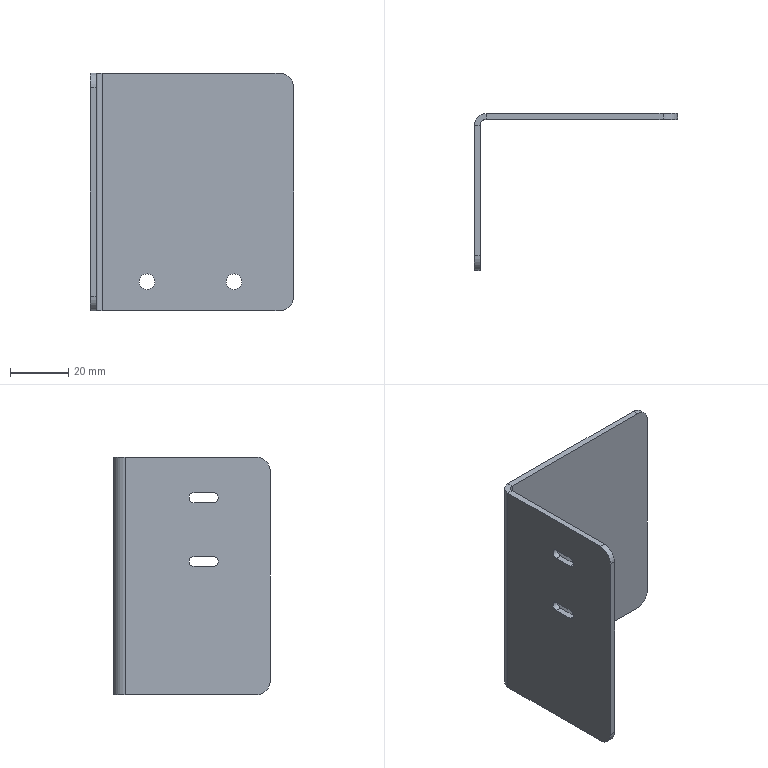Part | SolidWorks | features HoleWzd 3, EdgeFlange 2, Chamfer 1, Fillet 1, FlatPattern 1, MirrorPattern 1, SMBaseFlange 1, SheetMetal 1 | 1 solid | 30 faces | box 70 x 54 x 82 mm | volume 19533 mm3 | plane 16 | cylinder 14 | commonest cylinder face diameters 3.4 x4 5.5 x4 10 x4 4 x1 8 x1
STEP:
#1=CARTESIAN_POINT('',(47.503,28.,-28.25));
#2=VERTEX_POINT('',#1);
#3=CARTESIAN_POINT('',(47.503,28.,-33.75));
#4=VERTEX_POINT('',#3);
#5=CARTESIAN_POINT('',(47.503,28.,-31.));
#6=DIRECTION('',(0.,-1.,0.));
#7=DIRECTION('',(0.,0.,-1.));
#8=AXIS2_PLACEMENT_3D('',#5,#6,#7);
#9=CIRCLE('',#8,2.75);
#10=EDGE_CURVE('',#2,#4,#9,.T.);
#11=ORIENTED_EDGE('',*,*,#10,.F.);
#12=CARTESIAN_POINT('',(47.503,26.,-28.25));
#13=VERTEX_POINT('',#12);
#14=CARTESIAN_POINT('',(47.503,26.,-28.25));
#15=DIRECTION('',(0.,-1.,0.));
#16=VECTOR('',#15,1000.);
#17=LINE('',#14,#16);
#18=EDGE_CURVE('',#2,#13,#17,.T.);
#19=ORIENTED_EDGE('',*,*,#18,.T.);
#20=CARTESIAN_POINT('',(47.503,26.,-33.75));
#21=VERTEX_POINT('',#20);
#22=CARTESIAN_POINT('',(47.503,26.,-31.));
#23=DIRECTION('',(0.,-1.,0.));
#24=DIRECTION('',(0.,0.,-1.));
#25=AXIS2_PLACEMENT_3D('',#22,#23,#24);
#26=CIRCLE('',#25,2.75);
#27=EDGE_CURVE('',#13,#21,#26,.T.);
#28=ORIENTED_EDGE('',*,*,#27,.T.);
#29=CARTESIAN_POINT('',(47.503,26.,-33.75));
#30=DIRECTION('',(0.,-1.,0.));
#31=VECTOR('',#30,1000.);
#32=LINE('',#29,#31);
#33=EDGE_CURVE('',#4,#21,#32,.T.);
#34=ORIENTED_EDGE('',*,*,#33,.F.);
#35=EDGE_LOOP('',(#11,#19,#28,#34));
#36=FACE_OUTER_BOUND('',#35,.T.);
#37=CARTESIAN_POINT('',(47.503,26.,-31.));
#38=DIRECTION('',(0.,-1.,0.));
#39=DIRECTION('',(0.,0.,-1.));
#40=AXIS2_PLACEMENT_3D('',#37,#38,#39);
#41=CYLINDRICAL_SURFACE('',#40,2.75);
#42=ADVANCED_FACE('',(#36),#41,.F.);
#43=CARTESIAN_POINT('',(17.503,28.,-28.25));
#44=VERTEX_POINT('',#43);
#45=CARTESIAN_POINT('',(17.503,28.,-33.75));
#46=VERTEX_POINT('',#45);
#47=CARTESIAN_POINT('',(17.503,28.,-31.));
#48=DIRECTION('',(0.,-1.,0.));
#49=DIRECTION('',(0.,0.,-1.));
#50=AXIS2_PLACEMENT_3D('',#47,#48,#49);
#51=CIRCLE('',#50,2.75);
#52=EDGE_CURVE('',#44,#46,#51,.T.);
#53=ORIENTED_EDGE('',*,*,#52,.F.);
#54=CARTESIAN_POINT('',(17.503,26.,-28.25));
#55=VERTEX_POINT('',#54);
#56=CARTESIAN_POINT('',(17.503,26.,-28.25));
#57=DIRECTION('',(0.,-1.,0.));
#58=VECTOR('',#57,1000.);
#59=LINE('',#56,#58);
#60=EDGE_CURVE('',#44,#55,#59,.T.);
#61=ORIENTED_EDGE('',*,*,#60,.T.);
#62=CARTESIAN_POINT('',(17.503,26.,-33.75));
#63=VERTEX_POINT('',#62);
#64=CARTESIAN_POINT('',(17.503,26.,-31.));
#65=DIRECTION('',(0.,-1.,0.));
#66=DIRECTION('',(0.,0.,-1.));
#67=AXIS2_PLACEMENT_3D('',#64,#65,#66);
#68=CIRCLE('',#67,2.75);
#69=EDGE_CURVE('',#55,#63,#68,.T.);
#70=ORIENTED_EDGE('',*,*,#69,.T.);
#71=CARTESIAN_POINT('',(17.503,26.,-33.75));
#72=DIRECTION('',(0.,-1.,0.));
#73=VECTOR('',#72,1000.);
#74=LINE('',#71,#73);
#75=EDGE_CURVE('',#46,#63,#74,.T.);
#76=ORIENTED_EDGE('',*,*,#75,.F.);
#77=EDGE_LOOP('',(#53,#61,#70,#76));
#78=FACE_OUTER_BOUND('',#77,.T.);
#79=CARTESIAN_POINT('',(17.503,26.,-31.));
#80=DIRECTION('',(0.,-1.,0.));
#81=DIRECTION('',(0.,0.,-1.));
#82=AXIS2_PLACEMENT_3D('',#79,#80,#81);
#83=CYLINDRICAL_SURFACE('',#82,2.75);
#84=ADVANCED_FACE('',(#78),#83,.F.);
#85=CARTESIAN_POINT('',(-2.,24.,41.));
#86=VERTEX_POINT('',#85);
#87=CARTESIAN_POINT('',(-2.,-21.,41.));
#88=VERTEX_POINT('',#87);
#89=CARTESIAN_POINT('',(-2.,26.,41.));
#90=DIRECTION('',(0.,-1.,0.));
#91=VECTOR('',#90,1000.);
#92=LINE('',#89,#91);
#93=EDGE_CURVE('',#86,#88,#92,.T.);
#94=ORIENTED_EDGE('',*,*,#93,.T.);
#95=CARTESIAN_POINT('',(0.,-21.,41.));
#96=VERTEX_POINT('',#95);
#97=CARTESIAN_POINT('',(-2.,-21.,41.));
#98=DIRECTION('',(1.,0.,0.));
#99=VECTOR('',#98,1000.);
#100=LINE('',#97,#99);
#101=EDGE_CURVE('',#88,#96,#100,.T.);
#102=ORIENTED_EDGE('',*,*,#101,.T.);
#103=CARTESIAN_POINT('',(0.,24.,41.));
#104=VERTEX_POINT('',#103);
#105=CARTESIAN_POINT('',(0.,26.,41.));
#106=DIRECTION('',(0.,-1.,0.));
#107=VECTOR('',#106,1000.);
#108=LINE('',#105,#107);
#109=EDGE_CURVE('',#104,#96,#108,.T.);
#110=ORIENTED_EDGE('',*,*,#109,.F.);
#111=CARTESIAN_POINT('',(0.,24.,41.));
#112=DIRECTION('',(-1.,0.,0.));
#113=VECTOR('',#112,1000.);
#114=LINE('',#111,#113);
#115=EDGE_CURVE('',#104,#86,#114,.T.);
#116=ORIENTED_EDGE('',*,*,#115,.T.);
#117=EDGE_LOOP('',(#94,#102,#110,#116));
#118=FACE_OUTER_BOUND('',#117,.T.);
#119=CARTESIAN_POINT('',(-2.,26.,41.));
#120=DIRECTION('',(0.,0.,1.));
#121=DIRECTION('',(0.,-1.,0.));
#122=AXIS2_PLACEMENT_3D('',#119,#120,#121);
#123=PLANE('',#122);
#124=ADVANCED_FACE('',(#118),#123,.T.);
#125=CARTESIAN_POINT('',(-2.,-6.3,6.7));
#126=VERTEX_POINT('',#125);
#127=CARTESIAN_POINT('',(-2.,-6.3,3.3));
#128=VERTEX_POINT('',#127);
#129=CARTESIAN_POINT('',(-2.,-6.3,5.));
#130=DIRECTION('',(1.,0.,0.));
#131=DIRECTION('',(0.,0.,-1.));
#132=AXIS2_PLACEMENT_3D('',#129,#130,#131);
#133=CIRCLE('',#132,1.7);
#134=EDGE_CURVE('',#126,#128,#133,.T.);
#135=ORIENTED_EDGE('',*,*,#134,.T.);
#136=CARTESIAN_POINT('',(-2.,0.3,3.3));
#137=VERTEX_POINT('',#136);
#138=CARTESIAN_POINT('',(-2.,-6.3,3.3));
#139=DIRECTION('',(0.,1.,0.));
#140=VECTOR('',#139,1000.);
#141=LINE('',#138,#140);
#142=EDGE_CURVE('',#128,#137,#141,.T.);
#143=ORIENTED_EDGE('',*,*,#142,.T.);
#144=CARTESIAN_POINT('',(-2.,0.3,6.7));
#145=VERTEX_POINT('',#144);
#146=CARTESIAN_POINT('',(-2.,0.3,5.));
#147=DIRECTION('',(1.,0.,0.));
#148=DIRECTION('',(0.,0.,-1.));
#149=AXIS2_PLACEMENT_3D('',#146,#147,#148);
#150=CIRCLE('',#149,1.7);
#151=EDGE_CURVE('',#137,#145,#150,.T.);
#152=ORIENTED_EDGE('',*,*,#151,.T.);
#153=CARTESIAN_POINT('',(-2.,-6.3,6.7));
#154=DIRECTION('',(0.,1.,0.));
#155=VECTOR('',#154,1000.);
#156=LINE('',#153,#155);
#157=EDGE_CURVE('',#126,#145,#156,.T.);
#158=ORIENTED_EDGE('',*,*,#157,.F.);
#159=EDGE_LOOP('',(#135,#143,#152,#158));
#160=FACE_BOUND('',#159,.T.);
#161=CARTESIAN_POINT('',(-2.,-6.3,25.3));
#162=VERTEX_POINT('',#161);
#163=CARTESIAN_POINT('',(-2.,0.3,25.3));
#164=VERTEX_POINT('',#163);
#165=CARTESIAN_POINT('',(-2.,-6.3,25.3));
#166=DIRECTION('',(0.,1.,0.));
#167=VECTOR('',#166,1000.);
#168=LINE('',#165,#167);
#169=EDGE_CURVE('',#162,#164,#168,.T.);
#170=ORIENTED_EDGE('',*,*,#169,.T.);
#171=CARTESIAN_POINT('',(-2.,0.3,28.7));
#172=VERTEX_POINT('',#171);
#173=CARTESIAN_POINT('',(-2.,0.3,27.));
#174=DIRECTION('',(1.,0.,0.));
#175=DIRECTION('',(0.,0.,-1.));
#176=AXIS2_PLACEMENT_3D('',#173,#174,#175);
#177=CIRCLE('',#176,1.7);
#178=EDGE_CURVE('',#164,#172,#177,.T.);
#179=ORIENTED_EDGE('',*,*,#178,.T.);
#180=CARTESIAN_POINT('',(-2.,-6.3,28.7));
#181=VERTEX_POINT('',#180);
#182=CARTESIAN_POINT('',(-2.,-6.3,28.7));
#183=DIRECTION('',(0.,1.,0.));
#184=VECTOR('',#183,1000.);
#185=LINE('',#182,#184);
#186=EDGE_CURVE('',#181,#172,#185,.T.);
#187=ORIENTED_EDGE('',*,*,#186,.F.);
#188=CARTESIAN_POINT('',(-2.,-6.3,27.));
#189=DIRECTION('',(1.,0.,0.));
#190=DIRECTION('',(0.,0.,-1.));
#191=AXIS2_PLACEMENT_3D('',#188,#189,#190);
#192=CIRCLE('',#191,1.7);
#193=EDGE_CURVE('',#181,#162,#192,.T.);
#194=ORIENTED_EDGE('',*,*,#193,.T.);
#195=EDGE_LOOP('',(#170,#179,#187,#194));
#196=FACE_BOUND('',#195,.T.);
#197=CARTESIAN_POINT('',(-2.,-21.,-41.));
#198=VERTEX_POINT('',#197);
#199=CARTESIAN_POINT('',(-2.,24.,-41.));
#200=VERTEX_POINT('',#199);
#201=CARTESIAN_POINT('',(-2.,26.,-41.));
#202=DIRECTION('',(0.,1.,0.));
#203=VECTOR('',#202,1000.);
#204=LINE('',#201,#203);
#205=EDGE_CURVE('',#198,#200,#204,.T.);
#206=ORIENTED_EDGE('',*,*,#205,.F.);
#207=CARTESIAN_POINT('',(-2.,-26.,-36.));
#208=VERTEX_POINT('',#207);
#209=CARTESIAN_POINT('',(-2.,-21.,-36.));
#210=DIRECTION('',(-1.,0.,0.));
#211=DIRECTION('',(0.,0.,-1.));
#212=AXIS2_PLACEMENT_3D('',#209,#210,#211);
#213=CIRCLE('',#212,5.);
#214=EDGE_CURVE('',#198,#208,#213,.T.);
#215=ORIENTED_EDGE('',*,*,#214,.T.);
#216=CARTESIAN_POINT('',(-2.,-26.,36.));
#217=VERTEX_POINT('',#216);
#218=CARTESIAN_POINT('',(-2.,-26.,41.));
#219=DIRECTION('',(0.,0.,-1.));
#220=VECTOR('',#219,1000.);
#221=LINE('',#218,#220);
#222=EDGE_CURVE('',#217,#208,#221,.T.);
#223=ORIENTED_EDGE('',*,*,#222,.F.);
#224=CARTESIAN_POINT('',(-2.,-21.,36.));
#225=DIRECTION('',(-1.,0.,0.));
#226=DIRECTION('',(0.,0.,-1.));
#227=AXIS2_PLACEMENT_3D('',#224,#225,#226);
#228=CIRCLE('',#227,5.);
#229=EDGE_CURVE('',#217,#88,#228,.T.);
#230=ORIENTED_EDGE('',*,*,#229,.T.);
#231=ORIENTED_EDGE('',*,*,#93,.F.);
#232=CARTESIAN_POINT('',(-2.,24.,41.));
#233=DIRECTION('',(0.,0.,-1.));
#234=VECTOR('',#233,1000.);
#235=LINE('',#232,#234);
#236=EDGE_CURVE('',#86,#200,#235,.T.);
#237=ORIENTED_EDGE('',*,*,#236,.T.);
#238=EDGE_LOOP('',(#206,#215,#223,#230,#231,#237));
#239=FACE_OUTER_BOUND('',#238,.T.);
#240=CARTESIAN_POINT('',(-2.,0.,0.));
#241=DIRECTION('',(1.,0.,0.));
#242=DIRECTION('',(0.,0.,-1.));
#243=AXIS2_PLACEMENT_3D('',#240,#241,#242);
#244=PLANE('',#243);
#245=ADVANCED_FACE('',(#160,#196,#239),#244,.F.);
#246=CARTESIAN_POINT('',(0.,0.3,25.3));
#247=VERTEX_POINT('',#246);
#248=CARTESIAN_POINT('',(0.,0.3,28.7));
#249=VERTEX_POINT('',#248);
#250=CARTESIAN_POINT('',(0.,0.3,27.));
#251=DIRECTION('',(1.,0.,0.));
#252=DIRECTION('',(0.,0.,-1.));
#253=AXIS2_PLACEMENT_3D('',#250,#251,#252);
#254=CIRCLE('',#253,1.7);
#255=EDGE_CURVE('',#247,#249,#254,.T.);
#256=ORIENTED_EDGE('',*,*,#255,.F.);
#257=CARTESIAN_POINT('',(0.,-6.3,25.3));
#258=VERTEX_POINT('',#257);
#259=CARTESIAN_POINT('',(0.,-6.3,25.3));
#260=DIRECTION('',(0.,1.,0.));
#261=VECTOR('',#260,1000.);
#262=LINE('',#259,#261);
#263=EDGE_CURVE('',#258,#247,#262,.T.);
#264=ORIENTED_EDGE('',*,*,#263,.F.);
#265=CARTESIAN_POINT('',(0.,-6.3,28.7));
#266=VERTEX_POINT('',#265);
#267=CARTESIAN_POINT('',(0.,-6.3,27.));
#268=DIRECTION('',(1.,0.,0.));
#269=DIRECTION('',(0.,0.,-1.));
#270=AXIS2_PLACEMENT_3D('',#267,#268,#269);
#271=CIRCLE('',#270,1.7);
#272=EDGE_CURVE('',#266,#258,#271,.T.);
#273=ORIENTED_EDGE('',*,*,#272,.F.);
#274=CARTESIAN_POINT('',(0.,-6.3,28.7));
#275=DIRECTION('',(0.,1.,0.));
#276=VECTOR('',#275,1000.);
#277=LINE('',#274,#276);
#278=EDGE_CURVE('',#266,#249,#277,.T.);
#279=ORIENTED_EDGE('',*,*,#278,.T.);
#280=EDGE_LOOP('',(#256,#264,#273,#279));
#281=FACE_BOUND('',#280,.T.);
#282=CARTESIAN_POINT('',(0.,-6.3,3.3));
#283=VERTEX_POINT('',#282);
#284=CARTESIAN_POINT('',(0.,0.3,3.3));
#285=VERTEX_POINT('',#284);
#286=CARTESIAN_POINT('',(0.,-6.3,3.3));
#287=DIRECTION('',(0.,1.,0.));
#288=VECTOR('',#287,1000.);
#289=LINE('',#286,#288);
#290=EDGE_CURVE('',#283,#285,#289,.T.);
#291=ORIENTED_EDGE('',*,*,#290,.F.);
#292=CARTESIAN_POINT('',(0.,-6.3,6.7));
#293=VERTEX_POINT('',#292);
#294=CARTESIAN_POINT('',(0.,-6.3,5.));
#295=DIRECTION('',(1.,0.,0.));
#296=DIRECTION('',(0.,0.,-1.));
#297=AXIS2_PLACEMENT_3D('',#294,#295,#296);
#298=CIRCLE('',#297,1.7);
#299=EDGE_CURVE('',#293,#283,#298,.T.);
#300=ORIENTED_EDGE('',*,*,#299,.F.);
#301=CARTESIAN_POINT('',(0.,0.3,6.7));
#302=VERTEX_POINT('',#301);
#303=CARTESIAN_POINT('',(0.,-6.3,6.7));
#304=DIRECTION('',(0.,1.,0.));
#305=VECTOR('',#304,1000.);
#306=LINE('',#303,#305);
#307=EDGE_CURVE('',#293,#302,#306,.T.);
#308=ORIENTED_EDGE('',*,*,#307,.T.);
#309=CARTESIAN_POINT('',(0.,0.3,5.));
#310=DIRECTION('',(1.,0.,0.));
#311=DIRECTION('',(0.,0.,-1.));
#312=AXIS2_PLACEMENT_3D('',#309,#310,#311);
#313=CIRCLE('',#312,1.7);
#314=EDGE_CURVE('',#285,#302,#313,.T.);
#315=ORIENTED_EDGE('',*,*,#314,.F.);
#316=EDGE_LOOP('',(#291,#300,#308,#315));
#317=FACE_BOUND('',#316,.T.);
#318=CARTESIAN_POINT('',(0.,-26.,36.));
#319=VERTEX_POINT('',#318);
#320=CARTESIAN_POINT('',(0.,-26.,-36.));
#321=VERTEX_POINT('',#320);
#322=CARTESIAN_POINT('',(0.,-26.,41.));
#323=DIRECTION('',(0.,0.,-1.));
#324=VECTOR('',#323,1000.);
#325=LINE('',#322,#324);
#326=EDGE_CURVE('',#319,#321,#325,.T.);
#327=ORIENTED_EDGE('',*,*,#326,.T.);
#328=CARTESIAN_POINT('',(0.,-21.,-41.));
#329=VERTEX_POINT('',#328);
#330=CARTESIAN_POINT('',(0.,-21.,-36.));
#331=DIRECTION('',(1.,0.,0.));
#332=DIRECTION('',(0.,0.,-1.));
#333=AXIS2_PLACEMENT_3D('',#330,#331,#332);
#334=CIRCLE('',#333,5.);
#335=EDGE_CURVE('',#321,#329,#334,.T.);
#336=ORIENTED_EDGE('',*,*,#335,.T.);
#337=CARTESIAN_POINT('',(0.,24.,-41.));
#338=VERTEX_POINT('',#337);
#339=CARTESIAN_POINT('',(0.,26.,-41.));
#340=DIRECTION('',(0.,1.,0.));
#341=VECTOR('',#340,1000.);
#342=LINE('',#339,#341);
#343=EDGE_CURVE('',#329,#338,#342,.T.);
#344=ORIENTED_EDGE('',*,*,#343,.T.);
#345=CARTESIAN_POINT('',(0.,24.,41.));
#346=DIRECTION('',(0.,0.,-1.));
#347=VECTOR('',#346,1000.);
#348=LINE('',#345,#347);
#349=EDGE_CURVE('',#104,#338,#348,.T.);
#350=ORIENTED_EDGE('',*,*,#349,.F.);
#351=ORIENTED_EDGE('',*,*,#109,.T.);
#352=CARTESIAN_POINT('',(0.,-21.,36.));
#353=DIRECTION('',(1.,0.,0.));
#354=DIRECTION('',(0.,0.,-1.));
#355=AXIS2_PLACEMENT_3D('',#352,#353,#354);
#356=CIRCLE('',#355,5.);
#357=EDGE_CURVE('',#96,#319,#356,.T.);
#358=ORIENTED_EDGE('',*,*,#357,.T.);
#359=EDGE_LOOP('',(#327,#336,#344,#350,#351,#358));
#360=FACE_OUTER_BOUND('',#359,.T.);
#361=CARTESIAN_POINT('',(0.,0.,0.));
#362=DIRECTION('',(1.,0.,0.));
#363=DIRECTION('',(0.,0.,-1.));
#364=AXIS2_PLACEMENT_3D('',#361,#362,#363);
#365=PLANE('',#364);
#366=ADVANCED_FACE('',(#281,#317,#360),#365,.T.);
#367=ORIENTED_EDGE('',*,*,#343,.F.);
#368=CARTESIAN_POINT('',(-2.,-21.,-41.));
#369=DIRECTION('',(-1.,0.,0.));
#370=VECTOR('',#369,1000.);
#371=LINE('',#368,#370);
#372=EDGE_CURVE('',#329,#198,#371,.T.);
#373=ORIENTED_EDGE('',*,*,#372,.T.);
#374=ORIENTED_EDGE('',*,*,#205,.T.);
#375=CARTESIAN_POINT('',(0.,24.,-41.));
#376=DIRECTION('',(-1.,0.,0.));
#377=VECTOR('',#376,1000.);
#378=LINE('',#375,#377);
#379=EDGE_CURVE('',#338,#200,#378,.T.);
#380=ORIENTED_EDGE('',*,*,#379,.F.);
#381=EDGE_LOOP('',(#367,#373,#374,#380));
#382=FACE_OUTER_BOUND('',#381,.T.);
#383=CARTESIAN_POINT('',(-2.,26.,-41.));
#384=DIRECTION('',(0.,0.,-1.));
#385=DIRECTION('',(0.,1.,0.));
#386=AXIS2_PLACEMENT_3D('',#383,#384,#385);
#387=PLANE('',#386);
#388=ADVANCED_FACE('',(#382),#387,.T.);
#389=ORIENTED_EDGE('',*,*,#222,.T.);
#390=CARTESIAN_POINT('',(-2.,-26.,-36.));
#391=DIRECTION('',(1.,0.,0.));
#392=VECTOR('',#391,1000.);
#393=LINE('',#390,#392);
#394=EDGE_CURVE('',#208,#321,#393,.T.);
#395=ORIENTED_EDGE('',*,*,#394,.T.);
#396=ORIENTED_EDGE('',*,*,#326,.F.);
#397=CARTESIAN_POINT('',(-2.,-26.,36.));
#398=DIRECTION('',(-1.,0.,0.));
#399=VECTOR('',#398,1000.);
#400=LINE('',#397,#399);
#401=EDGE_CURVE('',#319,#217,#400,.T.);
#402=ORIENTED_EDGE('',*,*,#401,.T.);
#403=EDGE_LOOP('',(#389,#395,#396,#402));
#404=FACE_OUTER_BOUND('',#403,.T.);
#405=CARTESIAN_POINT('',(-2.,-26.,41.));
#406=DIRECTION('',(0.,-1.,0.));
#407=DIRECTION('',(0.,0.,-1.));
#408=AXIS2_PLACEMENT_3D('',#405,#406,#407);
#409=PLANE('',#408);
#410=ADVANCED_FACE('',(#404),#409,.T.);
#411=ORIENTED_EDGE('',*,*,#151,.F.);
#412=CARTESIAN_POINT('',(0.,0.3,3.3));
#413=DIRECTION('',(-1.,0.,0.));
#414=VECTOR('',#413,1000.);
#415=LINE('',#412,#414);
#416=EDGE_CURVE('',#285,#137,#415,.T.);
#417=ORIENTED_EDGE('',*,*,#416,.F.);
#418=ORIENTED_EDGE('',*,*,#314,.T.);
#419=CARTESIAN_POINT('',(0.,0.3,6.7));
#420=DIRECTION('',(1.,0.,0.));
#421=VECTOR('',#420,1000.);
#422=LINE('',#419,#421);
#423=EDGE_CURVE('',#145,#302,#422,.T.);
#424=ORIENTED_EDGE('',*,*,#423,.F.);
#425=EDGE_LOOP('',(#411,#417,#418,#424));
#426=FACE_OUTER_BOUND('',#425,.T.);
#427=CARTESIAN_POINT('',(0.,0.3,5.));
#428=DIRECTION('',(1.,0.,0.));
#429=DIRECTION('',(0.,0.,-1.));
#430=AXIS2_PLACEMENT_3D('',#427,#428,#429);
#431=CYLINDRICAL_SURFACE('',#430,1.7);
#432=ADVANCED_FACE('',(#426),#431,.F.);
#433=ORIENTED_EDGE('',*,*,#299,.T.);
#434=CARTESIAN_POINT('',(0.,-6.3,3.3));
#435=DIRECTION('',(1.,0.,0.));
#436=VECTOR('',#435,1000.);
#437=LINE('',#434,#436);
#438=EDGE_CURVE('',#128,#283,#437,.T.);
#439=ORIENTED_EDGE('',*,*,#438,.F.);
#440=ORIENTED_EDGE('',*,*,#134,.F.);
#441=CARTESIAN_POINT('',(0.,-6.3,6.7));
#442=DIRECTION('',(-1.,0.,0.));
#443=VECTOR('',#442,1000.);
#444=LINE('',#441,#443);
#445=EDGE_CURVE('',#293,#126,#444,.T.);
#446=ORIENTED_EDGE('',*,*,#445,.F.);
#447=EDGE_LOOP('',(#433,#439,#440,#446));
#448=FACE_OUTER_BOUND('',#447,.T.);
#449=CARTESIAN_POINT('',(0.,-6.3,5.));
#450=DIRECTION('',(1.,0.,0.));
#451=DIRECTION('',(0.,0.,-1.));
#452=AXIS2_PLACEMENT_3D('',#449,#450,#451);
#453=CYLINDRICAL_SURFACE('',#452,1.7);
#454=ADVANCED_FACE('',(#448),#453,.F.);
#455=ORIENTED_EDGE('',*,*,#423,.T.);
#456=ORIENTED_EDGE('',*,*,#307,.F.);
#457=ORIENTED_EDGE('',*,*,#445,.T.);
#458=ORIENTED_EDGE('',*,*,#157,.T.);
#459=EDGE_LOOP('',(#455,#456,#457,#458));
#460=FACE_OUTER_BOUND('',#459,.T.);
#461=CARTESIAN_POINT('',(0.,-6.3,6.7));
#462=DIRECTION('',(0.,0.,1.));
#463=DIRECTION('',(1.,0.,0.));
#464=AXIS2_PLACEMENT_3D('',#461,#462,#463);
#465=PLANE('',#464);
#466=ADVANCED_FACE('',(#460),#465,.F.);
#467=ORIENTED_EDGE('',*,*,#416,.T.);
#468=ORIENTED_EDGE('',*,*,#142,.F.);
#469=ORIENTED_EDGE('',*,*,#438,.T.);
#470=ORIENTED_EDGE('',*,*,#290,.T.);
#471=EDGE_LOOP('',(#467,#468,#469,#470));
#472=FACE_OUTER_BOUND('',#471,.T.);
#473=CARTESIAN_POINT('',(0.,-6.3,3.3));
#474=DIRECTION('',(0.,0.,-1.));
#475=DIRECTION('',(-1.,0.,0.));
#476=AXIS2_PLACEMENT_3D('',#473,#474,#475);
#477=PLANE('',#476);
#478=ADVANCED_FACE('',(#472),#477,.F.);
#479=ORIENTED_EDGE('',*,*,#178,.F.);
#480=CARTESIAN_POINT('',(0.,0.3,25.3));
#481=DIRECTION('',(-1.,0.,0.));
#482=VECTOR('',#481,1000.);
#483=LINE('',#480,#482);
#484=EDGE_CURVE('',#247,#164,#483,.T.);
#485=ORIENTED_EDGE('',*,*,#484,.F.);
#486=ORIENTED_EDGE('',*,*,#255,.T.);
#487=CARTESIAN_POINT('',(0.,0.3,28.7));
#488=DIRECTION('',(1.,0.,0.));
#489=VECTOR('',#488,1000.);
#490=LINE('',#487,#489);
#491=EDGE_CURVE('',#172,#249,#490,.T.);
#492=ORIENTED_EDGE('',*,*,#491,.F.);
#493=EDGE_LOOP('',(#479,#485,#486,#492));
#494=FACE_OUTER_BOUND('',#493,.T.);
#495=CARTESIAN_POINT('',(0.,0.3,27.));
#496=DIRECTION('',(1.,0.,0.));
#497=DIRECTION('',(0.,0.,-1.));
#498=AXIS2_PLACEMENT_3D('',#495,#496,#497);
#499=CYLINDRICAL_SURFACE('',#498,1.7);
#500=ADVANCED_FACE('',(#494),#499,.F.);
#501=ORIENTED_EDGE('',*,*,#272,.T.);
#502=CARTESIAN_POINT('',(0.,-6.3,25.3));
#503=DIRECTION('',(1.,0.,0.));
#504=VECTOR('',#503,1000.);
#505=LINE('',#502,#504);
#506=EDGE_CURVE('',#162,#258,#505,.T.);
#507=ORIENTED_EDGE('',*,*,#506,.F.);
#508=ORIENTED_EDGE('',*,*,#193,.F.);
#509=CARTESIAN_POINT('',(0.,-6.3,28.7));
#510=DIRECTION('',(-1.,0.,0.));
#511=VECTOR('',#510,1000.);
#512=LINE('',#509,#511);
#513=EDGE_CURVE('',#266,#181,#512,.T.);
#514=ORIENTED_EDGE('',*,*,#513,.F.);
#515=EDGE_LOOP('',(#501,#507,#508,#514));
#516=FACE_OUTER_BOUND('',#515,.T.);
#517=CARTESIAN_POINT('',(0.,-6.3,27.));
#518=DIRECTION('',(1.,0.,0.));
#519=DIRECTION('',(0.,0.,-1.));
#520=AXIS2_PLACEMENT_3D('',#517,#518,#519);
#521=CYLINDRICAL_SURFACE('',#520,1.7);
#522=ADVANCED_FACE('',(#516),#521,.F.);
#523=ORIENTED_EDGE('',*,*,#491,.T.);
#524=ORIENTED_EDGE('',*,*,#278,.F.);
#525=ORIENTED_EDGE('',*,*,#513,.T.);
#526=ORIENTED_EDGE('',*,*,#186,.T.);
#527=EDGE_LOOP('',(#523,#524,#525,#526));
#528=FACE_OUTER_BOUND('',#527,.T.);
#529=CARTESIAN_POINT('',(0.,-6.3,28.7));
#530=DIRECTION('',(0.,0.,1.));
#531=DIRECTION('',(1.,0.,0.));
#532=AXIS2_PLACEMENT_3D('',#529,#530,#531);
#533=PLANE('',#532);
#534=ADVANCED_FACE('',(#528),#533,.F.);
#535=ORIENTED_EDGE('',*,*,#484,.T.);
#536=ORIENTED_EDGE('',*,*,#169,.F.);
#537=ORIENTED_EDGE('',*,*,#506,.T.);
#538=ORIENTED_EDGE('',*,*,#263,.T.);
#539=EDGE_LOOP('',(#535,#536,#537,#538));
#540=FACE_OUTER_BOUND('',#539,.T.);
#541=CARTESIAN_POINT('',(0.,-6.3,25.3));
#542=DIRECTION('',(0.,0.,-1.));
#543=DIRECTION('',(-1.,0.,0.));
#544=AXIS2_PLACEMENT_3D('',#541,#542,#543);
#545=PLANE('',#544);
#546=ADVANCED_FACE('',(#540),#545,.F.);
#547=CARTESIAN_POINT('',(2.,26.,-41.));
#548=VERTEX_POINT('',#547);
#549=CARTESIAN_POINT('',(2.,28.,-41.));
#550=VERTEX_POINT('',#549);
#551=CARTESIAN_POINT('',(2.,26.,-41.));
#552=DIRECTION('',(0.,1.,0.));
#553=VECTOR('',#552,1000.);
#554=LINE('',#551,#553);
#555=EDGE_CURVE('',#548,#550,#554,.T.);
#556=ORIENTED_EDGE('',*,*,#555,.F.);
#557=CARTESIAN_POINT('',(2.,24.,-41.));
#558=DIRECTION('',(0.,0.,-1.));
#559=DIRECTION('',(1.,0.,0.));
#560=AXIS2_PLACEMENT_3D('',#557,#558,#559);
#561=CIRCLE('',#560,2.);
#562=EDGE_CURVE('',#338,#548,#561,.T.);
#563=ORIENTED_EDGE('',*,*,#562,.F.);
#564=ORIENTED_EDGE('',*,*,#379,.T.);
#565=CARTESIAN_POINT('',(2.,24.,-41.));
#566=DIRECTION('',(0.,0.,-1.));
#567=DIRECTION('',(1.,0.,0.));
#568=AXIS2_PLACEMENT_3D('',#565,#566,#567);
#569=CIRCLE('',#568,4.);
#570=EDGE_CURVE('',#200,#550,#569,.T.);
#571=ORIENTED_EDGE('',*,*,#570,.T.);
#572=EDGE_LOOP('',(#556,#563,#564,#571));
#573=FACE_OUTER_BOUND('',#572,.T.);
#574=CARTESIAN_POINT('',(2.,24.,-41.));
#575=DIRECTION('',(0.,0.,-1.));
#576=DIRECTION('',(-1.,0.,0.));
#577=AXIS2_PLACEMENT_3D('',#574,#575,#576);
#578=PLANE('',#577);
#579=ADVANCED_FACE('',(#573),#578,.T.);
#580=CARTESIAN_POINT('',(2.,26.,41.));
#581=VERTEX_POINT('',#580);
#582=CARTESIAN_POINT('',(2.,24.,41.));
#583=DIRECTION('',(0.,0.,1.));
#584=DIRECTION('',(1.,0.,0.));
#585=AXIS2_PLACEMENT_3D('',#582,#583,#584);
#586=CIRCLE('',#585,2.);
#587=EDGE_CURVE('',#581,#104,#586,.T.);
#588=ORIENTED_EDGE('',*,*,#587,.F.);
#589=CARTESIAN_POINT('',(2.,28.,41.));
#590=VERTEX_POINT('',#589);
#591=CARTESIAN_POINT('',(2.,26.,41.));
#592=DIRECTION('',(0.,1.,0.));
#593=VECTOR('',#592,1000.);
#594=LINE('',#591,#593);
#595=EDGE_CURVE('',#581,#590,#594,.T.);
#596=ORIENTED_EDGE('',*,*,#595,.T.);
#597=CARTESIAN_POINT('',(2.,24.,41.));
#598=DIRECTION('',(0.,0.,1.));
#599=DIRECTION('',(1.,0.,0.));
#600=AXIS2_PLACEMENT_3D('',#597,#598,#599);
#601=CIRCLE('',#600,4.);
#602=EDGE_CURVE('',#590,#86,#601,.T.);
#603=ORIENTED_EDGE('',*,*,#602,.T.);
#604=ORIENTED_EDGE('',*,*,#115,.F.);
#605=EDGE_LOOP('',(#588,#596,#603,#604));
#606=FACE_OUTER_BOUND('',#605,.T.);
#607=CARTESIAN_POINT('',(2.,24.,41.));
#608=DIRECTION('',(0.,0.,-1.));
#609=DIRECTION('',(-1.,0.,0.));
#610=AXIS2_PLACEMENT_3D('',#607,#608,#609);
#611=PLANE('',#610);
#612=ADVANCED_FACE('',(#606),#611,.F.);
#613=ORIENTED_EDGE('',*,*,#236,.F.);
#614=ORIENTED_EDGE('',*,*,#602,.F.);
#615=CARTESIAN_POINT('',(2.,28.,0.));
#616=DIRECTION('',(0.,0.,-1.));
#617=VECTOR('',#616,1000.);
#618=LINE('',#615,#617);
#619=EDGE_CURVE('',#590,#550,#618,.T.);
#620=ORIENTED_EDGE('',*,*,#619,.T.);
#621=ORIENTED_EDGE('',*,*,#570,.F.);
#622=EDGE_LOOP('',(#613,#614,#620,#621));
#623=FACE_OUTER_BOUND('',#622,.T.);
#624=CARTESIAN_POINT('',(2.,24.,41.));
#625=DIRECTION('',(0.,0.,1.));
#626=DIRECTION('',(0.,1.,0.));
#627=AXIS2_PLACEMENT_3D('',#624,#625,#626);
#628=CYLINDRICAL_SURFACE('',#627,4.);
#629=ADVANCED_FACE('',(#623),#628,.T.);
#630=ORIENTED_EDGE('',*,*,#349,.T.);
#631=ORIENTED_EDGE('',*,*,#562,.T.);
#632=CARTESIAN_POINT('',(2.,26.,-41.));
#633=DIRECTION('',(0.,0.,1.));
#634=VECTOR('',#633,1000.);
#635=LINE('',#632,#634);
#636=EDGE_CURVE('',#548,#581,#635,.T.);
#637=ORIENTED_EDGE('',*,*,#636,.T.);
#638=ORIENTED_EDGE('',*,*,#587,.T.);
#639=EDGE_LOOP('',(#630,#631,#637,#638));
#640=FACE_OUTER_BOUND('',#639,.T.);
#641=CARTESIAN_POINT('',(2.,24.,41.));
#642=DIRECTION('',(0.,0.,1.));
#643=DIRECTION('',(0.,1.,0.));
#644=AXIS2_PLACEMENT_3D('',#641,#642,#643);
#645=CYLINDRICAL_SURFACE('',#644,2.);
#646=ADVANCED_FACE('',(#640),#645,.F.);
#647=CARTESIAN_POINT('',(63.,28.,-41.));
#648=VERTEX_POINT('',#647);
#649=CARTESIAN_POINT('',(0.,28.,-41.));
#650=DIRECTION('',(-1.,0.,0.));
#651=VECTOR('',#650,1000.);
#652=LINE('',#649,#651);
#653=EDGE_CURVE('',#648,#550,#652,.T.);
#654=ORIENTED_EDGE('',*,*,#653,.F.);
#655=CARTESIAN_POINT('',(63.,26.,-41.));
#656=VERTEX_POINT('',#655);
#657=CARTESIAN_POINT('',(63.,28.,-41.));
#658=DIRECTION('',(0.,-1.,0.));
#659=VECTOR('',#658,1000.);
#660=LINE('',#657,#659);
#661=EDGE_CURVE('',#648,#656,#660,.T.);
#662=ORIENTED_EDGE('',*,*,#661,.T.);
#663=CARTESIAN_POINT('',(0.,26.,-41.));
#664=DIRECTION('',(-1.,0.,0.));
#665=VECTOR('',#664,1000.);
#666=LINE('',#663,#665);
#667=EDGE_CURVE('',#656,#548,#666,.T.);
#668=ORIENTED_EDGE('',*,*,#667,.T.);
#669=ORIENTED_EDGE('',*,*,#555,.T.);
#670=EDGE_LOOP('',(#654,#662,#668,#669));
#671=FACE_OUTER_BOUND('',#670,.T.);
#672=CARTESIAN_POINT('',(0.,28.,-41.));
#673=DIRECTION('',(0.,0.,1.));
#674=DIRECTION('',(1.,0.,0.));
#675=AXIS2_PLACEMENT_3D('',#672,#673,#674);
#676=PLANE('',#675);
#677=ADVANCED_FACE('',(#671),#676,.F.);
#678=CARTESIAN_POINT('',(63.,26.,41.));
#679=VERTEX_POINT('',#678);
#680=CARTESIAN_POINT('',(68.,26.,41.));
#681=DIRECTION('',(1.,0.,0.));
#682=VECTOR('',#681,1000.);
#683=LINE('',#680,#682);
#684=EDGE_CURVE('',#581,#679,#683,.T.);
#685=ORIENTED_EDGE('',*,*,#684,.T.);
#686=CARTESIAN_POINT('',(63.,28.,41.));
#687=VERTEX_POINT('',#686);
#688=CARTESIAN_POINT('',(63.,28.,41.));
#689=DIRECTION('',(0.,1.,0.));
#690=VECTOR('',#689,1000.);
#691=LINE('',#688,#690);
#692=EDGE_CURVE('',#679,#687,#691,.T.);
#693=ORIENTED_EDGE('',*,*,#692,.T.);
#694=CARTESIAN_POINT('',(68.,28.,41.));
#695=DIRECTION('',(1.,0.,0.));
#696=VECTOR('',#695,1000.);
#697=LINE('',#694,#696);
#698=EDGE_CURVE('',#590,#687,#697,.T.);
#699=ORIENTED_EDGE('',*,*,#698,.F.);
#700=ORIENTED_EDGE('',*,*,#595,.F.);
#701=EDGE_LOOP('',(#685,#693,#699,#700));
#702=FACE_OUTER_BOUND('',#701,.T.);
#703=CARTESIAN_POINT('',(68.,28.,41.));
#704=DIRECTION('',(0.,0.,-1.));
#705=DIRECTION('',(-1.,0.,0.));
#706=AXIS2_PLACEMENT_3D('',#703,#704,#705);
#707=PLANE('',#706);
#708=ADVANCED_FACE('',(#702),#707,.F.);
#709=CARTESIAN_POINT('',(47.503,28.,-31.));
#710=DIRECTION('',(0.,-1.,0.));
#711=DIRECTION('',(0.,0.,-1.));
#712=AXIS2_PLACEMENT_3D('',#709,#710,#711);
#713=CIRCLE('',#712,2.75);
#714=EDGE_CURVE('',#4,#2,#713,.T.);
#715=ORIENTED_EDGE('',*,*,#714,.T.);
#716=ORIENTED_EDGE('',*,*,#10,.T.);
#717=EDGE_LOOP('',(#715,#716));
#718=FACE_BOUND('',#717,.T.);
#719=CARTESIAN_POINT('',(17.503,28.,-31.));
#720=DIRECTION('',(0.,-1.,0.));
#721=DIRECTION('',(0.,0.,-1.));
#722=AXIS2_PLACEMENT_3D('',#719,#720,#721);
#723=CIRCLE('',#722,2.75);
#724=EDGE_CURVE('',#46,#44,#723,.T.);
#725=ORIENTED_EDGE('',*,*,#724,.T.);
#726=ORIENTED_EDGE('',*,*,#52,.T.);
#727=EDGE_LOOP('',(#725,#726));
#728=FACE_BOUND('',#727,.T.);
#729=ORIENTED_EDGE('',*,*,#698,.T.);
#730=CARTESIAN_POINT('',(68.,28.,36.));
#731=VERTEX_POINT('',#730);
#732=CARTESIAN_POINT('',(63.,28.,36.));
#733=DIRECTION('',(0.,1.,0.));
#734=DIRECTION('',(1.,0.,0.));
#735=AXIS2_PLACEMENT_3D('',#732,#733,#734);
#736=CIRCLE('',#735,5.);
#737=EDGE_CURVE('',#687,#731,#736,.T.);
#738=ORIENTED_EDGE('',*,*,#737,.T.);
#739=CARTESIAN_POINT('',(68.,28.,-36.));
#740=VERTEX_POINT('',#739);
#741=CARTESIAN_POINT('',(68.,28.,-41.));
#742=DIRECTION('',(0.,0.,-1.));
#743=VECTOR('',#742,1000.);
#744=LINE('',#741,#743);
#745=EDGE_CURVE('',#731,#740,#744,.T.);
#746=ORIENTED_EDGE('',*,*,#745,.T.);
#747=CARTESIAN_POINT('',(63.,28.,-36.));
#748=DIRECTION('',(0.,1.,0.));
#749=DIRECTION('',(1.,0.,0.));
#750=AXIS2_PLACEMENT_3D('',#747,#748,#749);
#751=CIRCLE('',#750,5.);
#752=EDGE_CURVE('',#740,#648,#751,.T.);
#753=ORIENTED_EDGE('',*,*,#752,.T.);
#754=ORIENTED_EDGE('',*,*,#653,.T.);
#755=ORIENTED_EDGE('',*,*,#619,.F.);
#756=EDGE_LOOP('',(#729,#738,#746,#753,#754,#755));
#757=FACE_OUTER_BOUND('',#756,.T.);
#758=CARTESIAN_POINT('',(0.,28.,0.));
#759=DIRECTION('',(0.,-1.,0.));
#760=DIRECTION('',(1.,0.,0.));
#761=AXIS2_PLACEMENT_3D('',#758,#759,#760);
#762=PLANE('',#761);
#763=ADVANCED_FACE('',(#718,#728,#757),#762,.F.);
#764=CARTESIAN_POINT('',(47.503,26.,-31.));
#765=DIRECTION('',(0.,-1.,0.));
#766=DIRECTION('',(0.,0.,-1.));
#767=AXIS2_PLACEMENT_3D('',#764,#765,#766);
#768=CIRCLE('',#767,2.75);
#769=EDGE_CURVE('',#21,#13,#768,.T.);
#770=ORIENTED_EDGE('',*,*,#769,.F.);
#771=ORIENTED_EDGE('',*,*,#27,.F.);
#772=EDGE_LOOP('',(#770,#771));
#773=FACE_BOUND('',#772,.T.);
#774=CARTESIAN_POINT('',(17.503,26.,-31.));
#775=DIRECTION('',(0.,-1.,0.));
#776=DIRECTION('',(0.,0.,-1.));
#777=AXIS2_PLACEMENT_3D('',#774,#775,#776);
#778=CIRCLE('',#777,2.75);
#779=EDGE_CURVE('',#63,#55,#778,.T.);
#780=ORIENTED_EDGE('',*,*,#779,.F.);
#781=ORIENTED_EDGE('',*,*,#69,.F.);
#782=EDGE_LOOP('',(#780,#781));
#783=FACE_BOUND('',#782,.T.);
#784=CARTESIAN_POINT('',(68.,26.,36.));
#785=VERTEX_POINT('',#784);
#786=CARTESIAN_POINT('',(68.,26.,-36.));
#787=VERTEX_POINT('',#786);
#788=CARTESIAN_POINT('',(68.,26.,-41.));
#789=DIRECTION('',(0.,0.,-1.));
#790=VECTOR('',#789,1000.);
#791=LINE('',#788,#790);
#792=EDGE_CURVE('',#785,#787,#791,.T.);
#793=ORIENTED_EDGE('',*,*,#792,.F.);
#794=CARTESIAN_POINT('',(63.,26.,36.));
#795=DIRECTION('',(0.,-1.,0.));
#796=DIRECTION('',(1.,0.,0.));
#797=AXIS2_PLACEMENT_3D('',#794,#795,#796);
#798=CIRCLE('',#797,5.);
#799=EDGE_CURVE('',#785,#679,#798,.T.);
#800=ORIENTED_EDGE('',*,*,#799,.T.);
#801=ORIENTED_EDGE('',*,*,#684,.F.);
#802=ORIENTED_EDGE('',*,*,#636,.F.);
#803=ORIENTED_EDGE('',*,*,#667,.F.);
#804=CARTESIAN_POINT('',(63.,26.,-36.));
#805=DIRECTION('',(0.,-1.,0.));
#806=DIRECTION('',(1.,0.,0.));
#807=AXIS2_PLACEMENT_3D('',#804,#805,#806);
#808=CIRCLE('',#807,5.);
#809=EDGE_CURVE('',#656,#787,#808,.T.);
#810=ORIENTED_EDGE('',*,*,#809,.T.);
#811=EDGE_LOOP('',(#793,#800,#801,#802,#803,#810));
#812=FACE_OUTER_BOUND('',#811,.T.);
#813=CARTESIAN_POINT('',(0.,26.,0.));
#814=DIRECTION('',(0.,-1.,0.));
#815=DIRECTION('',(1.,0.,0.));
#816=AXIS2_PLACEMENT_3D('',#813,#814,#815);
#817=PLANE('',#816);
#818=ADVANCED_FACE('',(#773,#783,#812),#817,.T.);
#819=ORIENTED_EDGE('',*,*,#745,.F.);
#820=CARTESIAN_POINT('',(68.,28.,36.));
#821=DIRECTION('',(0.,-1.,0.));
#822=VECTOR('',#821,1000.);
#823=LINE('',#820,#822);
#824=EDGE_CURVE('',#731,#785,#823,.T.);
#825=ORIENTED_EDGE('',*,*,#824,.T.);
#826=ORIENTED_EDGE('',*,*,#792,.T.);
#827=CARTESIAN_POINT('',(68.,28.,-36.));
#828=DIRECTION('',(0.,1.,0.));
#829=VECTOR('',#828,1000.);
#830=LINE('',#827,#829);
#831=EDGE_CURVE('',#787,#740,#830,.T.);
#832=ORIENTED_EDGE('',*,*,#831,.T.);
#833=EDGE_LOOP('',(#819,#825,#826,#832));
#834=FACE_OUTER_BOUND('',#833,.T.);
#835=CARTESIAN_POINT('',(68.,28.,-41.));
#836=DIRECTION('',(-1.,0.,0.));
#837=DIRECTION('',(0.,-1.,0.));
#838=AXIS2_PLACEMENT_3D('',#835,#836,#837);
#839=PLANE('',#838);
#840=ADVANCED_FACE('',(#834),#839,.F.);
#841=ORIENTED_EDGE('',*,*,#60,.F.);
#842=ORIENTED_EDGE('',*,*,#724,.F.);
#843=ORIENTED_EDGE('',*,*,#75,.T.);
#844=ORIENTED_EDGE('',*,*,#779,.T.);
#845=EDGE_LOOP('',(#841,#842,#843,#844));
#846=FACE_OUTER_BOUND('',#845,.T.);
#847=CARTESIAN_POINT('',(17.503,26.,-31.));
#848=DIRECTION('',(0.,-1.,0.));
#849=DIRECTION('',(0.,0.,-1.));
#850=AXIS2_PLACEMENT_3D('',#847,#848,#849);
#851=CYLINDRICAL_SURFACE('',#850,2.75);
#852=ADVANCED_FACE('',(#846),#851,.F.);
#853=ORIENTED_EDGE('',*,*,#18,.F.);
#854=ORIENTED_EDGE('',*,*,#714,.F.);
#855=ORIENTED_EDGE('',*,*,#33,.T.);
#856=ORIENTED_EDGE('',*,*,#769,.T.);
#857=EDGE_LOOP('',(#853,#854,#855,#856));
#858=FACE_OUTER_BOUND('',#857,.T.);
#859=CARTESIAN_POINT('',(47.503,26.,-31.));
#860=DIRECTION('',(0.,-1.,0.));
#861=DIRECTION('',(0.,0.,-1.));
#862=AXIS2_PLACEMENT_3D('',#859,#860,#861);
#863=CYLINDRICAL_SURFACE('',#862,2.75);
#864=ADVANCED_FACE('',(#858),#863,.F.);
#865=ORIENTED_EDGE('',*,*,#214,.F.);
#866=ORIENTED_EDGE('',*,*,#372,.F.);
#867=ORIENTED_EDGE('',*,*,#335,.F.);
#868=ORIENTED_EDGE('',*,*,#394,.F.);
#869=EDGE_LOOP('',(#865,#866,#867,#868));
#870=FACE_OUTER_BOUND('',#869,.T.);
#871=CARTESIAN_POINT('',(-2.,-21.,-36.));
#872=DIRECTION('',(1.,0.,0.));
#873=DIRECTION('',(0.,0.,-1.));
#874=AXIS2_PLACEMENT_3D('',#871,#872,#873);
#875=CYLINDRICAL_SURFACE('',#874,5.);
#876=ADVANCED_FACE('',(#870),#875,.T.);
#877=ORIENTED_EDGE('',*,*,#229,.F.);
#878=ORIENTED_EDGE('',*,*,#401,.F.);
#879=ORIENTED_EDGE('',*,*,#357,.F.);
#880=ORIENTED_EDGE('',*,*,#101,.F.);
#881=EDGE_LOOP('',(#877,#878,#879,#880));
#882=FACE_OUTER_BOUND('',#881,.T.);
#883=CARTESIAN_POINT('',(-2.,-21.,36.));
#884=DIRECTION('',(1.,0.,0.));
#885=DIRECTION('',(0.,0.,-1.));
#886=AXIS2_PLACEMENT_3D('',#883,#884,#885);
#887=CYLINDRICAL_SURFACE('',#886,5.);
#888=ADVANCED_FACE('',(#882),#887,.T.);
#889=ORIENTED_EDGE('',*,*,#737,.F.);
#890=ORIENTED_EDGE('',*,*,#692,.F.);
#891=ORIENTED_EDGE('',*,*,#799,.F.);
#892=ORIENTED_EDGE('',*,*,#824,.F.);
#893=EDGE_LOOP('',(#889,#890,#891,#892));
#894=FACE_OUTER_BOUND('',#893,.T.);
#895=CARTESIAN_POINT('',(63.,28.,36.));
#896=DIRECTION('',(0.,-1.,0.));
#897=DIRECTION('',(1.,0.,0.));
#898=AXIS2_PLACEMENT_3D('',#895,#896,#897);
#899=CYLINDRICAL_SURFACE('',#898,5.);
#900=ADVANCED_FACE('',(#894),#899,.T.);
#901=ORIENTED_EDGE('',*,*,#752,.F.);
#902=ORIENTED_EDGE('',*,*,#831,.F.);
#903=ORIENTED_EDGE('',*,*,#809,.F.);
#904=ORIENTED_EDGE('',*,*,#661,.F.);
#905=EDGE_LOOP('',(#901,#902,#903,#904));
#906=FACE_OUTER_BOUND('',#905,.T.);
#907=CARTESIAN_POINT('',(63.,28.,-36.));
#908=DIRECTION('',(0.,-1.,0.));
#909=DIRECTION('',(1.,0.,0.));
#910=AXIS2_PLACEMENT_3D('',#907,#908,#909);
#911=CYLINDRICAL_SURFACE('',#910,5.);
#912=ADVANCED_FACE('',(#906),#911,.T.);
#913=CLOSED_SHELL('',(#42,#84,#124,#245,#366,#388,#410,#432,#454,#466,#478,#500,#522,#534,#546,#579,#612,#629,#646,#677,#708,#763,#818,#840,#852,#864,#876,#888,#900,#912));
#914=MANIFOLD_SOLID_BREP('',#913);
#915=CARTESIAN_POINT('',(0.,0.,0.));
#916=DIRECTION('',(0.,0.,1.));
#917=DIRECTION('',(1.,0.,0.));
#918=AXIS2_PLACEMENT_3D('',#915,#916,#917);
#919=(LENGTH_UNIT()NAMED_UNIT(*)SI_UNIT(.MILLI.,.METRE.));
#920=UNCERTAINTY_MEASURE_WITH_UNIT(LENGTH_MEASURE(0.00001),#919,'','');
#921=(NAMED_UNIT(*)PLANE_ANGLE_UNIT()SI_UNIT($,.RADIAN.));
#922=(NAMED_UNIT(*)SI_UNIT($,.STERADIAN.)SOLID_ANGLE_UNIT());
#923=(GEOMETRIC_REPRESENTATION_CONTEXT(3)GLOBAL_UNCERTAINTY_ASSIGNED_CONTEXT((#920))GLOBAL_UNIT_ASSIGNED_CONTEXT((#919,#921,#922))REPRESENTATION_CONTEXT('',''));
#924=ADVANCED_BREP_SHAPE_REPRESENTATION('',(#914,#918),#923);